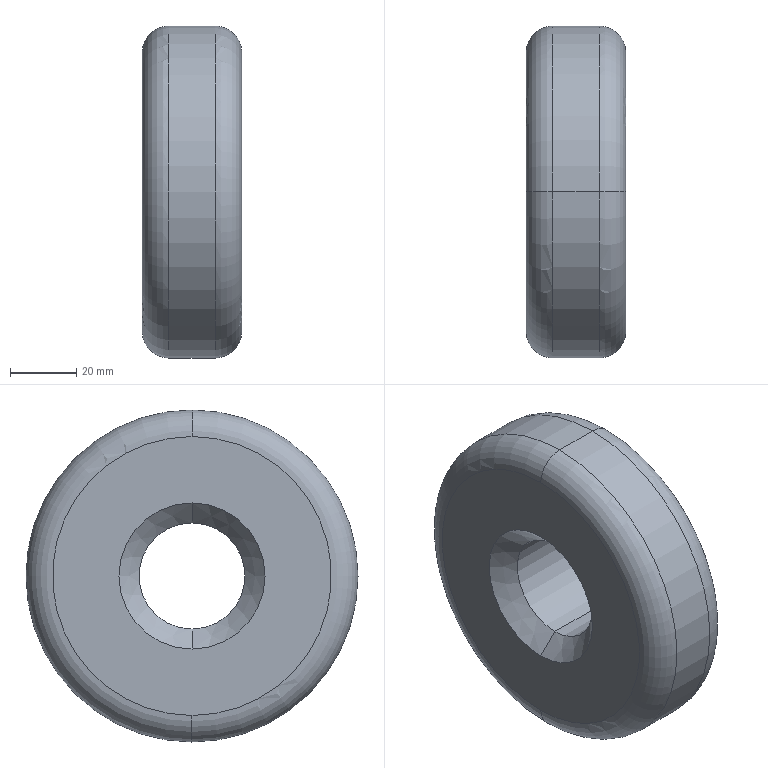Part | STEP file | 01-Support roller | 1 solid | 12 faces | box 30 x 100 x 100 mm | volume 201135 mm3 | cylinder 4 | torus 4 | cone 2 | plane 2 | commonest cylinder face diameters 32 x2 100 x2
STEP:
#1=CARTESIAN_POINT('',(0.,0.,0.));
#2=DIRECTION('',(0.,0.,1.));
#3=DIRECTION('',(1.,0.,0.));
#4=AXIS2_PLACEMENT_3D('',#1,#2,#3);
#5=CARTESIAN_POINT('',(6.,0.,16.));
#6=VERTEX_POINT('',#5);
#7=CARTESIAN_POINT('',(0.,0.,22.));
#8=VERTEX_POINT('',#7);
#9=CARTESIAN_POINT('',(6.,0.,16.));
#10=DIRECTION('',(-0.7071,0.,0.7071));
#11=VECTOR('',#10,1.);
#12=LINE('',#9,#11);
#13=CARTESIAN_POINT('',(6.,0.,0.));
#14=DIRECTION('',(-1.,0.,0.));
#15=DIRECTION('',(0.,0.,1.));
#16=AXIS2_PLACEMENT_3D('',#13,#14,#15);
#17=CONICAL_SURFACE('',#16,16.,0.7854);
#18=CARTESIAN_POINT('',(6.283,0.));
#19=DIRECTION('',(0.,1.));
#20=VECTOR('',#19,1.);
#21=LINE('',#18,#20);
#22=(GEOMETRIC_REPRESENTATION_CONTEXT(2)PARAMETRIC_REPRESENTATION_CONTEXT()REPRESENTATION_CONTEXT('',''));
#23=DEFINITIONAL_REPRESENTATION('',(#21),#22);
#24=PCURVE('',#17,#23);
#25=CARTESIAN_POINT('',(6.,0.,0.));
#26=DIRECTION('',(-1.,0.,0.));
#27=DIRECTION('',(0.,0.,1.));
#28=AXIS2_PLACEMENT_3D('',#25,#26,#27);
#29=CONICAL_SURFACE('',#28,16.,0.7854);
#30=CARTESIAN_POINT('',(0.,0.));
#31=DIRECTION('',(0.,1.));
#32=VECTOR('',#31,1.);
#33=LINE('',#30,#32);
#34=(GEOMETRIC_REPRESENTATION_CONTEXT(2)PARAMETRIC_REPRESENTATION_CONTEXT()REPRESENTATION_CONTEXT('',''));
#35=DEFINITIONAL_REPRESENTATION('',(#33),#34);
#36=PCURVE('',#29,#35);
#37=SURFACE_CURVE('',#12,(#24,#36),.PCURVE_S1.);
#38=EDGE_CURVE('',#6,#8,#37,.T.);
#39=ORIENTED_EDGE('',*,*,#38,.T.);
#40=CARTESIAN_POINT('',(0.,0.,-22.));
#41=VERTEX_POINT('',#40);
#42=CARTESIAN_POINT('',(0.,0.,0.));
#43=DIRECTION('',(1.,0.,0.));
#44=DIRECTION('',(0.,0.,-1.));
#45=AXIS2_PLACEMENT_3D('',#42,#43,#44);
#46=CIRCLE('',#45,22.);
#47=CARTESIAN_POINT('',(9.425,6.));
#48=DIRECTION('',(-1.,0.));
#49=VECTOR('',#48,1.);
#50=LINE('',#47,#49);
#51=(GEOMETRIC_REPRESENTATION_CONTEXT(2)PARAMETRIC_REPRESENTATION_CONTEXT()REPRESENTATION_CONTEXT('',''));
#52=DEFINITIONAL_REPRESENTATION('',(#50),#51);
#53=PCURVE('',#17,#52);
#54=CARTESIAN_POINT('',(0.,16.,0.));
#55=DIRECTION('',(1.,0.,0.));
#56=DIRECTION('',(0.,0.,-1.));
#57=AXIS2_PLACEMENT_3D('',#54,#55,#56);
#58=PLANE('',#57);
#59=CARTESIAN_POINT('',(0.,-16.));
#60=DIRECTION('',(1.,0.));
#61=AXIS2_PLACEMENT_2D('',#59,#60);
#62=CIRCLE('',#61,22.);
#63=(GEOMETRIC_REPRESENTATION_CONTEXT(2)PARAMETRIC_REPRESENTATION_CONTEXT()REPRESENTATION_CONTEXT('',''));
#64=DEFINITIONAL_REPRESENTATION('',(#62),#63);
#65=PCURVE('',#58,#64);
#66=SURFACE_CURVE('',#46,(#53,#65),.PCURVE_S1.);
#67=EDGE_CURVE('',#8,#41,#66,.T.);
#68=ORIENTED_EDGE('',*,*,#67,.T.);
#69=CARTESIAN_POINT('',(6.,0.,-16.));
#70=VERTEX_POINT('',#69);
#71=CARTESIAN_POINT('',(6.,0.,-16.));
#72=DIRECTION('',(-0.7071,0.,-0.7071));
#73=VECTOR('',#72,1.);
#74=LINE('',#71,#73);
#75=CARTESIAN_POINT('',(3.142,0.));
#76=DIRECTION('',(0.,1.));
#77=VECTOR('',#76,1.);
#78=LINE('',#75,#77);
#79=(GEOMETRIC_REPRESENTATION_CONTEXT(2)PARAMETRIC_REPRESENTATION_CONTEXT()REPRESENTATION_CONTEXT('',''));
#80=DEFINITIONAL_REPRESENTATION('',(#78),#79);
#81=PCURVE('',#17,#80);
#82=CARTESIAN_POINT('',(3.142,0.));
#83=DIRECTION('',(0.,1.));
#84=VECTOR('',#83,1.);
#85=LINE('',#82,#84);
#86=(GEOMETRIC_REPRESENTATION_CONTEXT(2)PARAMETRIC_REPRESENTATION_CONTEXT()REPRESENTATION_CONTEXT('',''));
#87=DEFINITIONAL_REPRESENTATION('',(#85),#86);
#88=PCURVE('',#29,#87);
#89=SURFACE_CURVE('',#74,(#81,#88),.PCURVE_S1.);
#90=EDGE_CURVE('',#70,#41,#89,.T.);
#91=ORIENTED_EDGE('',*,*,#90,.F.);
#92=CARTESIAN_POINT('',(6.,0.,0.));
#93=DIRECTION('',(-1.,0.,0.));
#94=DIRECTION('',(0.,0.,-1.));
#95=AXIS2_PLACEMENT_3D('',#92,#93,#94);
#96=CIRCLE('',#95,16.);
#97=CARTESIAN_POINT('',(3.142,0.));
#98=DIRECTION('',(1.,0.));
#99=VECTOR('',#98,1.);
#100=LINE('',#97,#99);
#101=(GEOMETRIC_REPRESENTATION_CONTEXT(2)PARAMETRIC_REPRESENTATION_CONTEXT()REPRESENTATION_CONTEXT('',''));
#102=DEFINITIONAL_REPRESENTATION('',(#100),#101);
#103=PCURVE('',#17,#102);
#104=CARTESIAN_POINT('',(0.,0.,0.));
#105=DIRECTION('',(-1.,0.,0.));
#106=DIRECTION('',(0.,0.,1.));
#107=AXIS2_PLACEMENT_3D('',#104,#105,#106);
#108=CYLINDRICAL_SURFACE('',#107,16.);
#109=CARTESIAN_POINT('',(3.142,-6.));
#110=DIRECTION('',(1.,0.));
#111=VECTOR('',#110,1.);
#112=LINE('',#109,#111);
#113=(GEOMETRIC_REPRESENTATION_CONTEXT(2)PARAMETRIC_REPRESENTATION_CONTEXT()REPRESENTATION_CONTEXT('',''));
#114=DEFINITIONAL_REPRESENTATION('',(#112),#113);
#115=PCURVE('',#108,#114);
#116=SURFACE_CURVE('',#96,(#103,#115),.PCURVE_S1.);
#117=EDGE_CURVE('',#70,#6,#116,.T.);
#118=ORIENTED_EDGE('',*,*,#117,.T.);
#119=EDGE_LOOP('',(#39,#68,#91,#118));
#120=FACE_BOUND('',#119,.F.);
#121=ADVANCED_FACE('',(#120),#17,.F.);
#122=CARTESIAN_POINT('',(30.,0.,16.));
#123=VERTEX_POINT('',#122);
#124=CARTESIAN_POINT('',(0.,0.,16.));
#125=DIRECTION('',(-1.,0.,0.));
#126=VECTOR('',#125,1.);
#127=LINE('',#124,#126);
#128=CARTESIAN_POINT('',(6.283,0.));
#129=DIRECTION('',(0.,1.));
#130=VECTOR('',#129,1.);
#131=LINE('',#128,#130);
#132=(GEOMETRIC_REPRESENTATION_CONTEXT(2)PARAMETRIC_REPRESENTATION_CONTEXT()REPRESENTATION_CONTEXT('',''));
#133=DEFINITIONAL_REPRESENTATION('',(#131),#132);
#134=PCURVE('',#108,#133);
#135=CARTESIAN_POINT('',(0.,0.,0.));
#136=DIRECTION('',(-1.,0.,0.));
#137=DIRECTION('',(0.,0.,1.));
#138=AXIS2_PLACEMENT_3D('',#135,#136,#137);
#139=CYLINDRICAL_SURFACE('',#138,16.);
#140=CARTESIAN_POINT('',(0.,0.));
#141=DIRECTION('',(0.,1.));
#142=VECTOR('',#141,1.);
#143=LINE('',#140,#142);
#144=(GEOMETRIC_REPRESENTATION_CONTEXT(2)PARAMETRIC_REPRESENTATION_CONTEXT()REPRESENTATION_CONTEXT('',''));
#145=DEFINITIONAL_REPRESENTATION('',(#143),#144);
#146=PCURVE('',#139,#145);
#147=SURFACE_CURVE('',#127,(#134,#146),.PCURVE_S1.);
#148=EDGE_CURVE('',#123,#6,#147,.T.);
#149=ORIENTED_EDGE('',*,*,#148,.T.);
#150=ORIENTED_EDGE('',*,*,#117,.F.);
#151=CARTESIAN_POINT('',(30.,0.,-16.));
#152=VERTEX_POINT('',#151);
#153=CARTESIAN_POINT('',(0.,0.,-16.));
#154=DIRECTION('',(-1.,0.,0.));
#155=VECTOR('',#154,1.);
#156=LINE('',#153,#155);
#157=CARTESIAN_POINT('',(3.142,0.));
#158=DIRECTION('',(0.,1.));
#159=VECTOR('',#158,1.);
#160=LINE('',#157,#159);
#161=(GEOMETRIC_REPRESENTATION_CONTEXT(2)PARAMETRIC_REPRESENTATION_CONTEXT()REPRESENTATION_CONTEXT('',''));
#162=DEFINITIONAL_REPRESENTATION('',(#160),#161);
#163=PCURVE('',#108,#162);
#164=CARTESIAN_POINT('',(3.142,0.));
#165=DIRECTION('',(0.,1.));
#166=VECTOR('',#165,1.);
#167=LINE('',#164,#166);
#168=(GEOMETRIC_REPRESENTATION_CONTEXT(2)PARAMETRIC_REPRESENTATION_CONTEXT()REPRESENTATION_CONTEXT('',''));
#169=DEFINITIONAL_REPRESENTATION('',(#167),#168);
#170=PCURVE('',#139,#169);
#171=SURFACE_CURVE('',#156,(#163,#170),.PCURVE_S1.);
#172=EDGE_CURVE('',#152,#70,#171,.T.);
#173=ORIENTED_EDGE('',*,*,#172,.F.);
#174=CARTESIAN_POINT('',(30.,0.,0.));
#175=DIRECTION('',(-1.,0.,0.));
#176=DIRECTION('',(0.,0.,1.));
#177=AXIS2_PLACEMENT_3D('',#174,#175,#176);
#178=CIRCLE('',#177,16.);
#179=CARTESIAN_POINT('',(0.,-30.));
#180=DIRECTION('',(1.,0.));
#181=VECTOR('',#180,1.);
#182=LINE('',#179,#181);
#183=(GEOMETRIC_REPRESENTATION_CONTEXT(2)PARAMETRIC_REPRESENTATION_CONTEXT()REPRESENTATION_CONTEXT('',''));
#184=DEFINITIONAL_REPRESENTATION('',(#182),#183);
#185=PCURVE('',#108,#184);
#186=CARTESIAN_POINT('',(30.,42.,0.));
#187=DIRECTION('',(-1.,0.,0.));
#188=DIRECTION('',(0.,0.,1.));
#189=AXIS2_PLACEMENT_3D('',#186,#187,#188);
#190=PLANE('',#189);
#191=CARTESIAN_POINT('',(0.,-42.));
#192=DIRECTION('',(1.,0.));
#193=AXIS2_PLACEMENT_2D('',#191,#192);
#194=CIRCLE('',#193,16.);
#195=(GEOMETRIC_REPRESENTATION_CONTEXT(2)PARAMETRIC_REPRESENTATION_CONTEXT()REPRESENTATION_CONTEXT('',''));
#196=DEFINITIONAL_REPRESENTATION('',(#194),#195);
#197=PCURVE('',#190,#196);
#198=SURFACE_CURVE('',#178,(#185,#197),.PCURVE_S1.);
#199=EDGE_CURVE('',#152,#123,#198,.T.);
#200=ORIENTED_EDGE('',*,*,#199,.T.);
#201=EDGE_LOOP('',(#149,#150,#173,#200));
#202=FACE_BOUND('',#201,.F.);
#203=ADVANCED_FACE('',(#202),#108,.F.);
#204=CARTESIAN_POINT('',(8.,0.,50.));
#205=VERTEX_POINT('',#204);
#206=CARTESIAN_POINT('',(8.,0.,-50.));
#207=VERTEX_POINT('',#206);
#208=CARTESIAN_POINT('',(8.,0.,0.));
#209=DIRECTION('',(-1.,0.,0.));
#210=DIRECTION('',(0.,0.,1.));
#211=AXIS2_PLACEMENT_3D('',#208,#209,#210);
#212=CIRCLE('',#211,50.);
#213=CARTESIAN_POINT('',(8.,0.,0.));
#214=DIRECTION('',(-1.,0.,0.));
#215=DIRECTION('',(0.,0.,1.));
#216=AXIS2_PLACEMENT_3D('',#213,#214,#215);
#217=TOROIDAL_SURFACE('',#216,42.,8.);
#218=CARTESIAN_POINT('',(0.,0.));
#219=DIRECTION('',(1.,0.));
#220=VECTOR('',#219,1.);
#221=LINE('',#218,#220);
#222=(GEOMETRIC_REPRESENTATION_CONTEXT(2)PARAMETRIC_REPRESENTATION_CONTEXT()REPRESENTATION_CONTEXT('',''));
#223=DEFINITIONAL_REPRESENTATION('',(#221),#222);
#224=PCURVE('',#217,#223);
#225=CARTESIAN_POINT('',(0.,0.,0.));
#226=DIRECTION('',(-1.,0.,0.));
#227=DIRECTION('',(0.,0.,1.));
#228=AXIS2_PLACEMENT_3D('',#225,#226,#227);
#229=CYLINDRICAL_SURFACE('',#228,50.);
#230=CARTESIAN_POINT('',(0.,-8.));
#231=DIRECTION('',(1.,0.));
#232=VECTOR('',#231,1.);
#233=LINE('',#230,#232);
#234=(GEOMETRIC_REPRESENTATION_CONTEXT(2)PARAMETRIC_REPRESENTATION_CONTEXT()REPRESENTATION_CONTEXT('',''));
#235=DEFINITIONAL_REPRESENTATION('',(#233),#234);
#236=PCURVE('',#229,#235);
#237=SURFACE_CURVE('',#212,(#224,#236),.PCURVE_S1.);
#238=EDGE_CURVE('',#205,#207,#237,.T.);
#239=ORIENTED_EDGE('',*,*,#238,.T.);
#240=CARTESIAN_POINT('',(0.,0.,-42.));
#241=VERTEX_POINT('',#240);
#242=CARTESIAN_POINT('',(8.,0.,-42.));
#243=DIRECTION('',(0.,1.,0.));
#244=DIRECTION('',(0.,0.,1.));
#245=AXIS2_PLACEMENT_3D('',#242,#243,#244);
#246=CIRCLE('',#245,8.);
#247=CARTESIAN_POINT('',(3.142,-3.142));
#248=DIRECTION('',(0.,1.));
#249=VECTOR('',#248,1.);
#250=LINE('',#247,#249);
#251=(GEOMETRIC_REPRESENTATION_CONTEXT(2)PARAMETRIC_REPRESENTATION_CONTEXT()REPRESENTATION_CONTEXT('',''));
#252=DEFINITIONAL_REPRESENTATION('',(#250),#251);
#253=PCURVE('',#217,#252);
#254=CARTESIAN_POINT('',(8.,0.,0.));
#255=DIRECTION('',(-1.,0.,0.));
#256=DIRECTION('',(0.,0.,1.));
#257=AXIS2_PLACEMENT_3D('',#254,#255,#256);
#258=TOROIDAL_SURFACE('',#257,42.,8.);
#259=CARTESIAN_POINT('',(3.142,-3.142));
#260=DIRECTION('',(0.,1.));
#261=VECTOR('',#260,1.);
#262=LINE('',#259,#261);
#263=(GEOMETRIC_REPRESENTATION_CONTEXT(2)PARAMETRIC_REPRESENTATION_CONTEXT()REPRESENTATION_CONTEXT('',''));
#264=DEFINITIONAL_REPRESENTATION('',(#262),#263);
#265=PCURVE('',#258,#264);
#266=SURFACE_CURVE('',#246,(#253,#265),.PCURVE_S1.);
#267=EDGE_CURVE('',#207,#241,#266,.T.);
#268=ORIENTED_EDGE('',*,*,#267,.T.);
#269=CARTESIAN_POINT('',(0.,0.,42.));
#270=VERTEX_POINT('',#269);
#271=CARTESIAN_POINT('',(0.,0.,0.));
#272=DIRECTION('',(-1.,0.,0.));
#273=DIRECTION('',(0.,0.,1.));
#274=AXIS2_PLACEMENT_3D('',#271,#272,#273);
#275=CIRCLE('',#274,42.);
#276=CARTESIAN_POINT('',(0.,1.571));
#277=DIRECTION('',(1.,0.));
#278=VECTOR('',#277,1.);
#279=LINE('',#276,#278);
#280=(GEOMETRIC_REPRESENTATION_CONTEXT(2)PARAMETRIC_REPRESENTATION_CONTEXT()REPRESENTATION_CONTEXT('',''));
#281=DEFINITIONAL_REPRESENTATION('',(#279),#280);
#282=PCURVE('',#217,#281);
#283=CARTESIAN_POINT('',(-42.,-16.));
#284=CARTESIAN_POINT('',(-42.,56.746));
#285=CARTESIAN_POINT('',(21.,20.373));
#286=CARTESIAN_POINT('',(84.,-16.));
#287=CARTESIAN_POINT('',(21.,-52.373));
#288=CARTESIAN_POINT('',(-42.,-88.746));
#289=CARTESIAN_POINT('',(-42.,-16.));
#290=(BOUNDED_CURVE()B_SPLINE_CURVE(2,(#283,#284,#285,#286,#287,#288,#289),.UNSPECIFIED.,.T.,.F.)B_SPLINE_CURVE_WITH_KNOTS((1,2,2,2,2,1),(-2.094,0.,2.094,4.189,6.283,8.378),.UNSPECIFIED.)CURVE()GEOMETRIC_REPRESENTATION_ITEM()RATIONAL_B_SPLINE_CURVE((1.,0.5,1.,0.5,1.,0.5,1.))REPRESENTATION_ITEM(''));
#291=(GEOMETRIC_REPRESENTATION_CONTEXT(2)PARAMETRIC_REPRESENTATION_CONTEXT()REPRESENTATION_CONTEXT('',''));
#292=DEFINITIONAL_REPRESENTATION('',(#290),#291);
#293=PCURVE('',#58,#292);
#294=SURFACE_CURVE('',#275,(#282,#293),.PCURVE_S1.);
#295=EDGE_CURVE('',#270,#241,#294,.T.);
#296=ORIENTED_EDGE('',*,*,#295,.F.);
#297=CARTESIAN_POINT('',(8.,0.,42.));
#298=DIRECTION('',(0.,-1.,0.));
#299=DIRECTION('',(0.,0.,-1.));
#300=AXIS2_PLACEMENT_3D('',#297,#298,#299);
#301=CIRCLE('',#300,8.);
#302=CARTESIAN_POINT('',(0.,-3.142));
#303=DIRECTION('',(0.,1.));
#304=VECTOR('',#303,1.);
#305=LINE('',#302,#304);
#306=(GEOMETRIC_REPRESENTATION_CONTEXT(2)PARAMETRIC_REPRESENTATION_CONTEXT()REPRESENTATION_CONTEXT('',''));
#307=DEFINITIONAL_REPRESENTATION('',(#305),#306);
#308=PCURVE('',#217,#307);
#309=CARTESIAN_POINT('',(6.283,-3.142));
#310=DIRECTION('',(0.,1.));
#311=VECTOR('',#310,1.);
#312=LINE('',#309,#311);
#313=(GEOMETRIC_REPRESENTATION_CONTEXT(2)PARAMETRIC_REPRESENTATION_CONTEXT()REPRESENTATION_CONTEXT('',''));
#314=DEFINITIONAL_REPRESENTATION('',(#312),#313);
#315=PCURVE('',#258,#314);
#316=SURFACE_CURVE('',#301,(#308,#315),.PCURVE_S1.);
#317=EDGE_CURVE('',#205,#270,#316,.T.);
#318=ORIENTED_EDGE('',*,*,#317,.F.);
#319=EDGE_LOOP('',(#239,#268,#296,#318));
#320=FACE_BOUND('',#319,.T.);
#321=ADVANCED_FACE('',(#320),#217,.T.);
#322=CARTESIAN_POINT('',(22.,0.,50.));
#323=VERTEX_POINT('',#322);
#324=CARTESIAN_POINT('',(22.,0.,-50.));
#325=VERTEX_POINT('',#324);
#326=CARTESIAN_POINT('',(22.,0.,0.));
#327=DIRECTION('',(-1.,0.,0.));
#328=DIRECTION('',(0.,0.,1.));
#329=AXIS2_PLACEMENT_3D('',#326,#327,#328);
#330=CIRCLE('',#329,50.);
#331=CARTESIAN_POINT('',(0.,-22.));
#332=DIRECTION('',(1.,0.));
#333=VECTOR('',#332,1.);
#334=LINE('',#331,#333);
#335=(GEOMETRIC_REPRESENTATION_CONTEXT(2)PARAMETRIC_REPRESENTATION_CONTEXT()REPRESENTATION_CONTEXT('',''));
#336=DEFINITIONAL_REPRESENTATION('',(#334),#335);
#337=PCURVE('',#229,#336);
#338=CARTESIAN_POINT('',(22.,0.,0.));
#339=DIRECTION('',(-1.,0.,0.));
#340=DIRECTION('',(0.,0.,1.));
#341=AXIS2_PLACEMENT_3D('',#338,#339,#340);
#342=TOROIDAL_SURFACE('',#341,42.,8.);
#343=CARTESIAN_POINT('',(0.,6.283));
#344=DIRECTION('',(1.,0.));
#345=VECTOR('',#344,1.);
#346=LINE('',#343,#345);
#347=(GEOMETRIC_REPRESENTATION_CONTEXT(2)PARAMETRIC_REPRESENTATION_CONTEXT()REPRESENTATION_CONTEXT('',''));
#348=DEFINITIONAL_REPRESENTATION('',(#346),#347);
#349=PCURVE('',#342,#348);
#350=SURFACE_CURVE('',#330,(#337,#349),.PCURVE_S1.);
#351=EDGE_CURVE('',#323,#325,#350,.T.);
#352=ORIENTED_EDGE('',*,*,#351,.T.);
#353=CARTESIAN_POINT('',(0.,0.,-50.));
#354=DIRECTION('',(-1.,0.,0.));
#355=VECTOR('',#354,1.);
#356=LINE('',#353,#355);
#357=CARTESIAN_POINT('',(3.142,0.));
#358=DIRECTION('',(0.,1.));
#359=VECTOR('',#358,1.);
#360=LINE('',#357,#359);
#361=(GEOMETRIC_REPRESENTATION_CONTEXT(2)PARAMETRIC_REPRESENTATION_CONTEXT()REPRESENTATION_CONTEXT('',''));
#362=DEFINITIONAL_REPRESENTATION('',(#360),#361);
#363=PCURVE('',#229,#362);
#364=CARTESIAN_POINT('',(0.,0.,0.));
#365=DIRECTION('',(-1.,0.,0.));
#366=DIRECTION('',(0.,0.,1.));
#367=AXIS2_PLACEMENT_3D('',#364,#365,#366);
#368=CYLINDRICAL_SURFACE('',#367,50.);
#369=CARTESIAN_POINT('',(3.142,0.));
#370=DIRECTION('',(0.,1.));
#371=VECTOR('',#370,1.);
#372=LINE('',#369,#371);
#373=(GEOMETRIC_REPRESENTATION_CONTEXT(2)PARAMETRIC_REPRESENTATION_CONTEXT()REPRESENTATION_CONTEXT('',''));
#374=DEFINITIONAL_REPRESENTATION('',(#372),#373);
#375=PCURVE('',#368,#374);
#376=SURFACE_CURVE('',#356,(#363,#375),.PCURVE_S1.);
#377=EDGE_CURVE('',#325,#207,#376,.T.);
#378=ORIENTED_EDGE('',*,*,#377,.T.);
#379=ORIENTED_EDGE('',*,*,#238,.F.);
#380=CARTESIAN_POINT('',(0.,0.,50.));
#381=DIRECTION('',(-1.,0.,0.));
#382=VECTOR('',#381,1.);
#383=LINE('',#380,#382);
#384=CARTESIAN_POINT('',(0.,0.));
#385=DIRECTION('',(0.,1.));
#386=VECTOR('',#385,1.);
#387=LINE('',#384,#386);
#388=(GEOMETRIC_REPRESENTATION_CONTEXT(2)PARAMETRIC_REPRESENTATION_CONTEXT()REPRESENTATION_CONTEXT('',''));
#389=DEFINITIONAL_REPRESENTATION('',(#387),#388);
#390=PCURVE('',#229,#389);
#391=CARTESIAN_POINT('',(6.283,0.));
#392=DIRECTION('',(0.,1.));
#393=VECTOR('',#392,1.);
#394=LINE('',#391,#393);
#395=(GEOMETRIC_REPRESENTATION_CONTEXT(2)PARAMETRIC_REPRESENTATION_CONTEXT()REPRESENTATION_CONTEXT('',''));
#396=DEFINITIONAL_REPRESENTATION('',(#394),#395);
#397=PCURVE('',#368,#396);
#398=SURFACE_CURVE('',#383,(#390,#397),.PCURVE_S1.);
#399=EDGE_CURVE('',#323,#205,#398,.T.);
#400=ORIENTED_EDGE('',*,*,#399,.F.);
#401=EDGE_LOOP('',(#352,#378,#379,#400));
#402=FACE_BOUND('',#401,.T.);
#403=ADVANCED_FACE('',(#402),#229,.T.);
#404=CARTESIAN_POINT('',(30.,0.,42.));
#405=VERTEX_POINT('',#404);
#406=CARTESIAN_POINT('',(30.,0.,-42.));
#407=VERTEX_POINT('',#406);
#408=CARTESIAN_POINT('',(30.,0.,0.));
#409=DIRECTION('',(-1.,0.,0.));
#410=DIRECTION('',(0.,0.,1.));
#411=AXIS2_PLACEMENT_3D('',#408,#409,#410);
#412=CIRCLE('',#411,42.);
#413=CARTESIAN_POINT('',(0.,4.712));
#414=DIRECTION('',(1.,0.));
#415=VECTOR('',#414,1.);
#416=LINE('',#413,#415);
#417=(GEOMETRIC_REPRESENTATION_CONTEXT(2)PARAMETRIC_REPRESENTATION_CONTEXT()REPRESENTATION_CONTEXT('',''));
#418=DEFINITIONAL_REPRESENTATION('',(#416),#417);
#419=PCURVE('',#342,#418);
#420=CARTESIAN_POINT('',(0.,-42.));
#421=DIRECTION('',(1.,0.));
#422=AXIS2_PLACEMENT_2D('',#420,#421);
#423=CIRCLE('',#422,42.);
#424=(GEOMETRIC_REPRESENTATION_CONTEXT(2)PARAMETRIC_REPRESENTATION_CONTEXT()REPRESENTATION_CONTEXT('',''));
#425=DEFINITIONAL_REPRESENTATION('',(#423),#424);
#426=PCURVE('',#190,#425);
#427=SURFACE_CURVE('',#412,(#419,#426),.PCURVE_S1.);
#428=EDGE_CURVE('',#405,#407,#427,.T.);
#429=ORIENTED_EDGE('',*,*,#428,.T.);
#430=CARTESIAN_POINT('',(22.,0.,-42.));
#431=DIRECTION('',(0.,1.,0.));
#432=DIRECTION('',(0.,0.,1.));
#433=AXIS2_PLACEMENT_3D('',#430,#431,#432);
#434=CIRCLE('',#433,8.);
#435=CARTESIAN_POINT('',(3.142,3.142));
#436=DIRECTION('',(0.,1.));
#437=VECTOR('',#436,1.);
#438=LINE('',#435,#437);
#439=(GEOMETRIC_REPRESENTATION_CONTEXT(2)PARAMETRIC_REPRESENTATION_CONTEXT()REPRESENTATION_CONTEXT('',''));
#440=DEFINITIONAL_REPRESENTATION('',(#438),#439);
#441=PCURVE('',#342,#440);
#442=CARTESIAN_POINT('',(22.,0.,0.));
#443=DIRECTION('',(-1.,0.,0.));
#444=DIRECTION('',(0.,0.,1.));
#445=AXIS2_PLACEMENT_3D('',#442,#443,#444);
#446=TOROIDAL_SURFACE('',#445,42.,8.);
#447=CARTESIAN_POINT('',(3.142,3.142));
#448=DIRECTION('',(0.,1.));
#449=VECTOR('',#448,1.);
#450=LINE('',#447,#449);
#451=(GEOMETRIC_REPRESENTATION_CONTEXT(2)PARAMETRIC_REPRESENTATION_CONTEXT()REPRESENTATION_CONTEXT('',''));
#452=DEFINITIONAL_REPRESENTATION('',(#450),#451);
#453=PCURVE('',#446,#452);
#454=SURFACE_CURVE('',#434,(#441,#453),.PCURVE_S1.);
#455=EDGE_CURVE('',#407,#325,#454,.T.);
#456=ORIENTED_EDGE('',*,*,#455,.T.);
#457=ORIENTED_EDGE('',*,*,#351,.F.);
#458=CARTESIAN_POINT('',(22.,0.,42.));
#459=DIRECTION('',(0.,-1.,0.));
#460=DIRECTION('',(0.,0.,-1.));
#461=AXIS2_PLACEMENT_3D('',#458,#459,#460);
#462=CIRCLE('',#461,8.);
#463=CARTESIAN_POINT('',(0.,3.142));
#464=DIRECTION('',(0.,1.));
#465=VECTOR('',#464,1.);
#466=LINE('',#463,#465);
#467=(GEOMETRIC_REPRESENTATION_CONTEXT(2)PARAMETRIC_REPRESENTATION_CONTEXT()REPRESENTATION_CONTEXT('',''));
#468=DEFINITIONAL_REPRESENTATION('',(#466),#467);
#469=PCURVE('',#342,#468);
#470=CARTESIAN_POINT('',(6.283,3.142));
#471=DIRECTION('',(0.,1.));
#472=VECTOR('',#471,1.);
#473=LINE('',#470,#472);
#474=(GEOMETRIC_REPRESENTATION_CONTEXT(2)PARAMETRIC_REPRESENTATION_CONTEXT()REPRESENTATION_CONTEXT('',''));
#475=DEFINITIONAL_REPRESENTATION('',(#473),#474);
#476=PCURVE('',#446,#475);
#477=SURFACE_CURVE('',#462,(#469,#476),.PCURVE_S1.);
#478=EDGE_CURVE('',#405,#323,#477,.T.);
#479=ORIENTED_EDGE('',*,*,#478,.F.);
#480=EDGE_LOOP('',(#429,#456,#457,#479));
#481=FACE_BOUND('',#480,.T.);
#482=ADVANCED_FACE('',(#481),#342,.T.);
#483=ORIENTED_EDGE('',*,*,#455,.F.);
#484=CARTESIAN_POINT('',(30.,0.,0.));
#485=DIRECTION('',(-1.,0.,0.));
#486=DIRECTION('',(0.,0.,1.));
#487=AXIS2_PLACEMENT_3D('',#484,#485,#486);
#488=CIRCLE('',#487,42.);
#489=CARTESIAN_POINT('',(0.,4.712));
#490=DIRECTION('',(1.,0.));
#491=VECTOR('',#490,1.);
#492=LINE('',#489,#491);
#493=(GEOMETRIC_REPRESENTATION_CONTEXT(2)PARAMETRIC_REPRESENTATION_CONTEXT()REPRESENTATION_CONTEXT('',''));
#494=DEFINITIONAL_REPRESENTATION('',(#492),#493);
#495=PCURVE('',#446,#494);
#496=CARTESIAN_POINT('',(0.,-42.));
#497=DIRECTION('',(1.,0.));
#498=AXIS2_PLACEMENT_2D('',#496,#497);
#499=CIRCLE('',#498,42.);
#500=(GEOMETRIC_REPRESENTATION_CONTEXT(2)PARAMETRIC_REPRESENTATION_CONTEXT()REPRESENTATION_CONTEXT('',''));
#501=DEFINITIONAL_REPRESENTATION('',(#499),#500);
#502=PCURVE('',#190,#501);
#503=SURFACE_CURVE('',#488,(#495,#502),.PCURVE_S1.);
#504=EDGE_CURVE('',#407,#405,#503,.T.);
#505=ORIENTED_EDGE('',*,*,#504,.T.);
#506=ORIENTED_EDGE('',*,*,#478,.T.);
#507=CARTESIAN_POINT('',(22.,0.,0.));
#508=DIRECTION('',(-1.,0.,0.));
#509=DIRECTION('',(0.,0.,1.));
#510=AXIS2_PLACEMENT_3D('',#507,#508,#509);
#511=CIRCLE('',#510,50.);
#512=CARTESIAN_POINT('',(0.,6.283));
#513=DIRECTION('',(1.,0.));
#514=VECTOR('',#513,1.);
#515=LINE('',#512,#514);
#516=(GEOMETRIC_REPRESENTATION_CONTEXT(2)PARAMETRIC_REPRESENTATION_CONTEXT()REPRESENTATION_CONTEXT('',''));
#517=DEFINITIONAL_REPRESENTATION('',(#515),#516);
#518=PCURVE('',#446,#517);
#519=CARTESIAN_POINT('',(0.,-22.));
#520=DIRECTION('',(1.,0.));
#521=VECTOR('',#520,1.);
#522=LINE('',#519,#521);
#523=(GEOMETRIC_REPRESENTATION_CONTEXT(2)PARAMETRIC_REPRESENTATION_CONTEXT()REPRESENTATION_CONTEXT('',''));
#524=DEFINITIONAL_REPRESENTATION('',(#522),#523);
#525=PCURVE('',#368,#524);
#526=SURFACE_CURVE('',#511,(#518,#525),.PCURVE_S1.);
#527=EDGE_CURVE('',#325,#323,#526,.T.);
#528=ORIENTED_EDGE('',*,*,#527,.F.);
#529=EDGE_LOOP('',(#483,#505,#506,#528));
#530=FACE_BOUND('',#529,.T.);
#531=ADVANCED_FACE('',(#530),#446,.T.);
#532=ORIENTED_EDGE('',*,*,#377,.F.);
#533=ORIENTED_EDGE('',*,*,#527,.T.);
#534=ORIENTED_EDGE('',*,*,#399,.T.);
#535=CARTESIAN_POINT('',(8.,0.,0.));
#536=DIRECTION('',(-1.,0.,0.));
#537=DIRECTION('',(0.,0.,1.));
#538=AXIS2_PLACEMENT_3D('',#535,#536,#537);
#539=CIRCLE('',#538,50.);
#540=CARTESIAN_POINT('',(0.,-8.));
#541=DIRECTION('',(1.,0.));
#542=VECTOR('',#541,1.);
#543=LINE('',#540,#542);
#544=(GEOMETRIC_REPRESENTATION_CONTEXT(2)PARAMETRIC_REPRESENTATION_CONTEXT()REPRESENTATION_CONTEXT('',''));
#545=DEFINITIONAL_REPRESENTATION('',(#543),#544);
#546=PCURVE('',#368,#545);
#547=CARTESIAN_POINT('',(0.,0.));
#548=DIRECTION('',(1.,0.));
#549=VECTOR('',#548,1.);
#550=LINE('',#547,#549);
#551=(GEOMETRIC_REPRESENTATION_CONTEXT(2)PARAMETRIC_REPRESENTATION_CONTEXT()REPRESENTATION_CONTEXT('',''));
#552=DEFINITIONAL_REPRESENTATION('',(#550),#551);
#553=PCURVE('',#258,#552);
#554=SURFACE_CURVE('',#539,(#546,#553),.PCURVE_S1.);
#555=EDGE_CURVE('',#207,#205,#554,.T.);
#556=ORIENTED_EDGE('',*,*,#555,.F.);
#557=EDGE_LOOP('',(#532,#533,#534,#556));
#558=FACE_BOUND('',#557,.T.);
#559=ADVANCED_FACE('',(#558),#368,.T.);
#560=ORIENTED_EDGE('',*,*,#267,.F.);
#561=ORIENTED_EDGE('',*,*,#555,.T.);
#562=ORIENTED_EDGE('',*,*,#317,.T.);
#563=CARTESIAN_POINT('',(0.,0.,0.));
#564=DIRECTION('',(-1.,0.,0.));
#565=DIRECTION('',(0.,0.,1.));
#566=AXIS2_PLACEMENT_3D('',#563,#564,#565);
#567=CIRCLE('',#566,42.);
#568=CARTESIAN_POINT('',(0.,1.571));
#569=DIRECTION('',(1.,0.));
#570=VECTOR('',#569,1.);
#571=LINE('',#568,#570);
#572=(GEOMETRIC_REPRESENTATION_CONTEXT(2)PARAMETRIC_REPRESENTATION_CONTEXT()REPRESENTATION_CONTEXT('',''));
#573=DEFINITIONAL_REPRESENTATION('',(#571),#572);
#574=PCURVE('',#258,#573);
#575=CARTESIAN_POINT('',(-42.,-16.));
#576=CARTESIAN_POINT('',(-42.,56.746));
#577=CARTESIAN_POINT('',(21.,20.373));
#578=CARTESIAN_POINT('',(84.,-16.));
#579=CARTESIAN_POINT('',(21.,-52.373));
#580=CARTESIAN_POINT('',(-42.,-88.746));
#581=CARTESIAN_POINT('',(-42.,-16.));
#582=(BOUNDED_CURVE()B_SPLINE_CURVE(2,(#575,#576,#577,#578,#579,#580,#581),.UNSPECIFIED.,.T.,.F.)B_SPLINE_CURVE_WITH_KNOTS((1,2,2,2,2,1),(-2.094,0.,2.094,4.189,6.283,8.378),.UNSPECIFIED.)CURVE()GEOMETRIC_REPRESENTATION_ITEM()RATIONAL_B_SPLINE_CURVE((1.,0.5,1.,0.5,1.,0.5,1.))REPRESENTATION_ITEM(''));
#583=(GEOMETRIC_REPRESENTATION_CONTEXT(2)PARAMETRIC_REPRESENTATION_CONTEXT()REPRESENTATION_CONTEXT('',''));
#584=DEFINITIONAL_REPRESENTATION('',(#582),#583);
#585=PCURVE('',#58,#584);
#586=SURFACE_CURVE('',#567,(#574,#585),.PCURVE_S1.);
#587=EDGE_CURVE('',#241,#270,#586,.T.);
#588=ORIENTED_EDGE('',*,*,#587,.F.);
#589=EDGE_LOOP('',(#560,#561,#562,#588));
#590=FACE_BOUND('',#589,.T.);
#591=ADVANCED_FACE('',(#590),#258,.T.);
#592=ORIENTED_EDGE('',*,*,#67,.T.);
#593=CARTESIAN_POINT('',(0.,0.,0.));
#594=DIRECTION('',(1.,0.,0.));
#595=DIRECTION('',(0.,0.,-1.));
#596=AXIS2_PLACEMENT_3D('',#593,#594,#595);
#597=CIRCLE('',#596,22.);
#598=CARTESIAN_POINT('',(0.,-16.));
#599=DIRECTION('',(1.,0.));
#600=AXIS2_PLACEMENT_2D('',#598,#599);
#601=CIRCLE('',#600,22.);
#602=(GEOMETRIC_REPRESENTATION_CONTEXT(2)PARAMETRIC_REPRESENTATION_CONTEXT()REPRESENTATION_CONTEXT('',''));
#603=DEFINITIONAL_REPRESENTATION('',(#601),#602);
#604=PCURVE('',#58,#603);
#605=CARTESIAN_POINT('',(3.142,6.));
#606=DIRECTION('',(-1.,0.));
#607=VECTOR('',#606,1.);
#608=LINE('',#605,#607);
#609=(GEOMETRIC_REPRESENTATION_CONTEXT(2)PARAMETRIC_REPRESENTATION_CONTEXT()REPRESENTATION_CONTEXT('',''));
#610=DEFINITIONAL_REPRESENTATION('',(#608),#609);
#611=PCURVE('',#29,#610);
#612=SURFACE_CURVE('',#597,(#604,#611),.PCURVE_S1.);
#613=EDGE_CURVE('',#41,#8,#612,.T.);
#614=ORIENTED_EDGE('',*,*,#613,.T.);
#615=EDGE_LOOP('',(#592,#614));
#616=FACE_BOUND('',#615,.T.);
#617=ORIENTED_EDGE('',*,*,#295,.T.);
#618=ORIENTED_EDGE('',*,*,#587,.T.);
#619=EDGE_LOOP('',(#617,#618));
#620=FACE_BOUND('',#619,.T.);
#621=ADVANCED_FACE('',(#616,#620),#58,.F.);
#622=CARTESIAN_POINT('',(6.,0.,0.));
#623=DIRECTION('',(-1.,0.,0.));
#624=DIRECTION('',(0.,0.,-1.));
#625=AXIS2_PLACEMENT_3D('',#622,#623,#624);
#626=CIRCLE('',#625,16.);
#627=CARTESIAN_POINT('',(-3.142,-6.));
#628=DIRECTION('',(1.,0.));
#629=VECTOR('',#628,1.);
#630=LINE('',#627,#629);
#631=(GEOMETRIC_REPRESENTATION_CONTEXT(2)PARAMETRIC_REPRESENTATION_CONTEXT()REPRESENTATION_CONTEXT('',''));
#632=DEFINITIONAL_REPRESENTATION('',(#630),#631);
#633=PCURVE('',#139,#632);
#634=CARTESIAN_POINT('',(-3.142,0.));
#635=DIRECTION('',(1.,0.));
#636=VECTOR('',#635,1.);
#637=LINE('',#634,#636);
#638=(GEOMETRIC_REPRESENTATION_CONTEXT(2)PARAMETRIC_REPRESENTATION_CONTEXT()REPRESENTATION_CONTEXT('',''));
#639=DEFINITIONAL_REPRESENTATION('',(#637),#638);
#640=PCURVE('',#29,#639);
#641=SURFACE_CURVE('',#626,(#633,#640),.PCURVE_S1.);
#642=EDGE_CURVE('',#6,#70,#641,.T.);
#643=ORIENTED_EDGE('',*,*,#642,.F.);
#644=ORIENTED_EDGE('',*,*,#148,.F.);
#645=CARTESIAN_POINT('',(30.,0.,0.));
#646=DIRECTION('',(-1.,0.,0.));
#647=DIRECTION('',(0.,0.,1.));
#648=AXIS2_PLACEMENT_3D('',#645,#646,#647);
#649=CIRCLE('',#648,16.);
#650=CARTESIAN_POINT('',(0.,-30.));
#651=DIRECTION('',(1.,0.));
#652=VECTOR('',#651,1.);
#653=LINE('',#650,#652);
#654=(GEOMETRIC_REPRESENTATION_CONTEXT(2)PARAMETRIC_REPRESENTATION_CONTEXT()REPRESENTATION_CONTEXT('',''));
#655=DEFINITIONAL_REPRESENTATION('',(#653),#654);
#656=PCURVE('',#139,#655);
#657=CARTESIAN_POINT('',(0.,-42.));
#658=DIRECTION('',(1.,0.));
#659=AXIS2_PLACEMENT_2D('',#657,#658);
#660=CIRCLE('',#659,16.);
#661=(GEOMETRIC_REPRESENTATION_CONTEXT(2)PARAMETRIC_REPRESENTATION_CONTEXT()REPRESENTATION_CONTEXT('',''));
#662=DEFINITIONAL_REPRESENTATION('',(#660),#661);
#663=PCURVE('',#190,#662);
#664=SURFACE_CURVE('',#649,(#656,#663),.PCURVE_S1.);
#665=EDGE_CURVE('',#123,#152,#664,.T.);
#666=ORIENTED_EDGE('',*,*,#665,.T.);
#667=ORIENTED_EDGE('',*,*,#172,.T.);
#668=EDGE_LOOP('',(#643,#644,#666,#667));
#669=FACE_BOUND('',#668,.F.);
#670=ADVANCED_FACE('',(#669),#139,.F.);
#671=ORIENTED_EDGE('',*,*,#428,.F.);
#672=ORIENTED_EDGE('',*,*,#504,.F.);
#673=EDGE_LOOP('',(#671,#672));
#674=FACE_BOUND('',#673,.T.);
#675=ORIENTED_EDGE('',*,*,#665,.T.);
#676=ORIENTED_EDGE('',*,*,#199,.T.);
#677=EDGE_LOOP('',(#675,#676));
#678=FACE_BOUND('',#677,.T.);
#679=ADVANCED_FACE('',(#674,#678),#190,.F.);
#680=ORIENTED_EDGE('',*,*,#613,.T.);
#681=ORIENTED_EDGE('',*,*,#38,.F.);
#682=ORIENTED_EDGE('',*,*,#642,.T.);
#683=ORIENTED_EDGE('',*,*,#90,.T.);
#684=EDGE_LOOP('',(#680,#681,#682,#683));
#685=FACE_BOUND('',#684,.F.);
#686=ADVANCED_FACE('',(#685),#29,.F.);
#687=CLOSED_SHELL('',(#121,#203,#321,#403,#482,#531,#559,#591,#621,#670,#679,#686));
#688=MANIFOLD_SOLID_BREP('',#687);
#689=(LENGTH_UNIT()NAMED_UNIT(*)SI_UNIT(.MILLI.,.METRE.));
#690=UNCERTAINTY_MEASURE_WITH_UNIT(LENGTH_MEASURE(0.0000001),#689,'','');
#691=(NAMED_UNIT(*)PLANE_ANGLE_UNIT()SI_UNIT($,.RADIAN.));
#692=(NAMED_UNIT(*)SI_UNIT($,.STERADIAN.)SOLID_ANGLE_UNIT());
#693=(GEOMETRIC_REPRESENTATION_CONTEXT(3)GLOBAL_UNCERTAINTY_ASSIGNED_CONTEXT((#690))GLOBAL_UNIT_ASSIGNED_CONTEXT((#689,#691,#692))REPRESENTATION_CONTEXT('',''));
#694=ADVANCED_BREP_SHAPE_REPRESENTATION('',(#4,#688),#693);